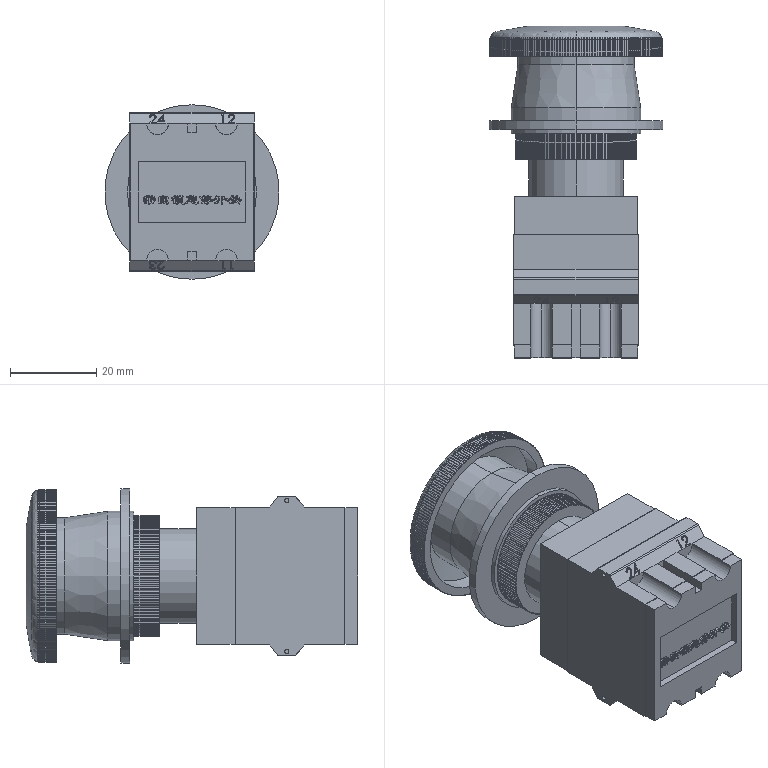Part | SolidWorks | features BaseBody 1 | 1 solid | 1374 faces | box 40.5 x 77 x 40.5 mm | volume 60164 mm3 | cylinder 720 | spline 399 | plane 249 | cone 6 | commonest cylinder face diameters 0.2 x239 40 x200 0.5 x145 28 x100 1 x12 5 x6